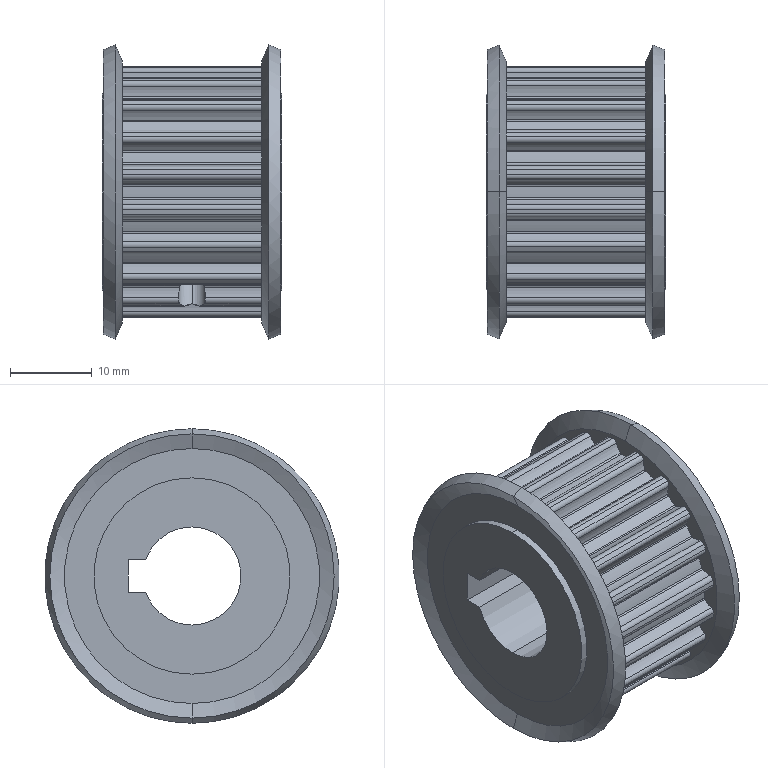Part | STEP file | 1 solid | 216 faces | box 22 x 36 x 36 mm | volume 12348 mm3 | cylinder 195 | cone 12 | plane 9 | commonest cylinder face diameters 1.1 x53 0.5 x45 6.55 x43 27.33 x22 30.87 x21 3.242 x4